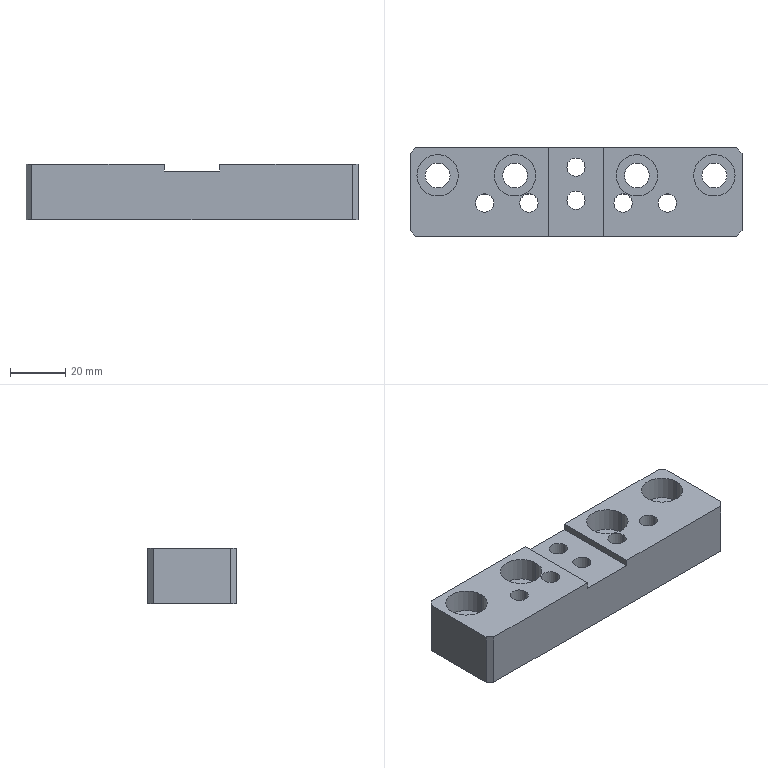Part | STEP file | PN_0022 | 1 solid | 64 faces | box 120 x 32 x 20 mm | volume 59836 mm3 | cylinder 40 | plane 24 | commonest cylinder face diameters 6.6 x12 11 x12 9 x8 15 x8